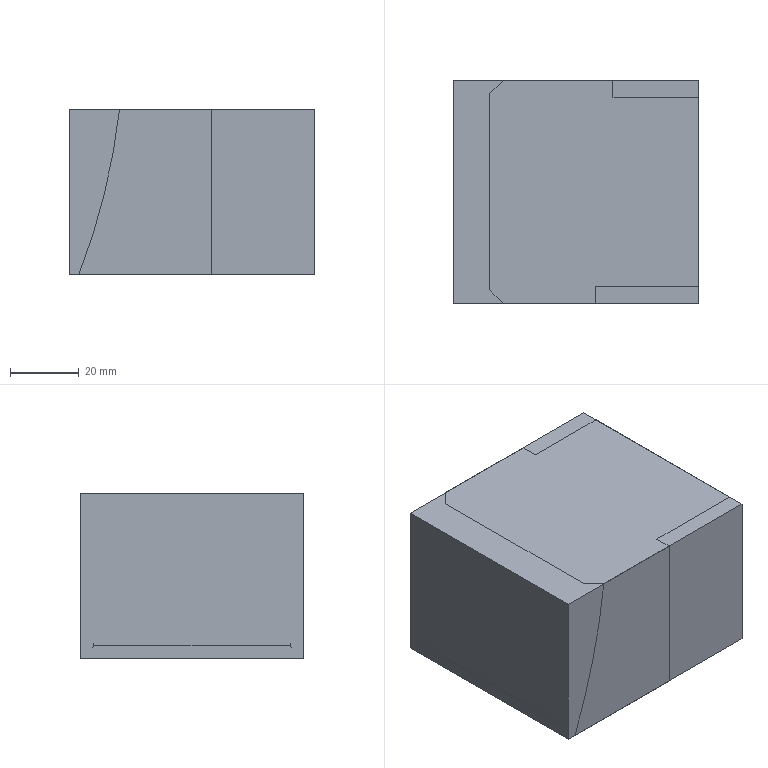NC program | NX | posted with a generic post | part box 71.51 x 65 x 48 mm
Lines 1 to 1113 of 48030:
N10 G17 G21 G94 G90
(FIXED_CONTOUR_COPY , TOOL : D6R0.5)
N12 T05 M6
N14 G54
N16 G17 G0 G90 X29.161 Y-29.75 B0. C0. S9500 M3
N18 G43 Z101.51 H5
N20 Z64.31
N22 G94 G1 Z60.474 F500.
N24 X29.148 Y-29.766
N26 X29.13 Y-29.777
N28 X29.109 Y-29.78
N30 X29.003 Z60.476 F3500.
N32 X28.925 Z60.478
N34 X28.771 Z60.481
N36 X28.616 Z60.482
N38 X28.46
N40 X27.842 Z60.481
N42 X-28.151
N44 X-28.306
N46 X-28.615 Z60.48
N48 X-28.77 Z60.479
N50 X-28.935 Z60.476
N52 X-28.999 Y-29.768
N54 X-29.072 Y-29.752
N56 X-29.124 Y-29.74
N58 X-29.079 Z60.477
N60 X-28.924 Z60.481
N62 X-28.77 Z60.483
N64 X-28.601 Z60.485
N66 X-28.306 Z60.486
N68 X-27.687
N70 X27.842
N72 X28.461 Z60.487
N74 X28.616
N76 X28.771 Z60.485
N78 X28.925 Z60.483
N80 X29.08 Z60.479
N82 X29.235 Z60.474
N84 X29.262 Z60.473
N86 X29.292 Y-29.731
N88 X29.388 Y-29.696
N90 X29.413 Y-29.687
N92 X29.389 Z60.475
N94 X29.235 Z60.481
N96 X29.08 Z60.485
N98 X28.925 Z60.489
N100 X28.771 Z60.491
N102 X28.616 Z60.493
N104 X28.461
N106 X27.842 Z60.492
N108 X-28.151
N110 X-28.306
N112 X-28.645 Z60.491
N114 X-28.77 Z60.489
N116 X-28.924 Z60.487
N118 X-29.079 Z60.483
N120 X-29.234 Z60.478
N122 X-29.306 Z60.476
N124 X-29.381 Y-29.661
N126 X-29.459 Y-29.631
N128 X-29.475 Y-29.624
N130 X-29.388 Z60.48
N132 X-29.234 Z60.486
N134 X-29.078 Z60.491
N136 X-28.924 Z60.494
N138 X-28.758 Z60.497
N140 X-28.652 Z60.498
N142 X-28.306 Z60.499
N144 X-25.977
N146 X27.842
N148 X28.461 Z60.5
N150 X28.616
N152 X28.771 Z60.499
N154 X28.931 Z60.496
N156 X29.086 Z60.493
N158 X29.234 Z60.488
N160 X29.389 Z60.482
N162 X29.544 Z60.474
N164 X29.569 Z60.473
N166 X29.691 Y-29.568
N168 X29.721 Y-29.552
N170 X29.699 Z60.474
N172 X29.544 Z60.483
N174 X29.389 Z60.49
N176 X29.235 Z60.496
N178 X29.08 Z60.501
N180 X28.925 Z60.505
N182 X28.771 Z60.507
N184 X28.616 Z60.509
N186 X28.461
N188 X27.842 Z60.508
N190 X-28.306
N192 X-28.619 Z60.507
N194 X-28.693 Z60.506
N196 X-28.77 Z60.505
N198 X-28.924 Z60.503
N200 X-29.079 Z60.499
N202 X-29.234 Z60.494
N204 X-29.388 Z60.488
N206 X-29.543 Z60.481
N208 X-29.635 Z60.476
N210 X-29.69 Y-29.524
N212 X-29.768 Y-29.482
N214 X-29.784 Y-29.472
N216 X-29.698 Z60.481
N218 X-29.542 Z60.49
N220 X-29.388 Z60.498
N222 X-29.234 Z60.504
N224 X-29.079 Z60.509
N226 X-28.924 Z60.512
N228 X-28.77 Z60.515
N230 X-28.657 Z60.516
N232 X-28.538
N234 X-28.46
N236 X-28.306 Z60.517
N238 X27.842
N240 X28.461 Z60.518
N242 X28.616
N244 X28.771 Z60.516
N246 X28.925 Z60.514
N248 X29.08 Z60.51
N250 X29.235 Z60.506
N252 X29.389 Z60.5
N254 X29.549 Z60.492
N256 X29.698 Z60.483
N258 X29.861 Z60.473
N260 X29.938 Y-29.422 Z60.472
N262 X29.988 Y-29.387 Z60.473
N264 X29.853 Z60.483
N266 X29.699 Z60.493
N268 X29.544 Z60.502
N270 X29.389 Z60.509
N272 X29.235 Z60.516
N274 X29.08 Z60.52
N276 X28.925 Z60.524
N278 X28.771 Z60.526
N280 X28.616 Z60.528
N282 X28.461
N284 X27.842 Z60.527
N286 X-28.306 Y-29.388
N288 X-28.46 Z60.526
N290 X-28.538
N292 X-28.655
N294 X-28.77 Z60.525
N296 X-28.924 Z60.522
N298 X-29.079 Z60.519
N300 X-29.234 Z60.514
N302 X-29.388 Z60.508
N304 X-29.543 Z60.5
N306 X-29.698 Z60.491
N308 X-29.852 Z60.481
N310 X-29.921 Z60.476
N312 X-29.935 Y-29.379
N314 X-30.002 Y-29.331
N316 X-30.046 Y-29.299
N318 X-30.007 Z60.479
N320 X-29.852 Z60.491
N322 X-29.698 Z60.502
N324 X-29.543 Z60.511
N326 X-29.388 Z60.518
N328 X-29.234 Z60.524
N330 X-29.079 Z60.529
N332 X-28.924 Z60.533
N334 X-28.77 Z60.535
N336 X-28.654 Z60.536
N338 X-28.541 Z60.537
N340 X-28.46
N342 X-28.311
N344 X27.838
N346 X28.461 Z60.538
N348 X28.616
N350 X28.771 Z60.537
N352 X28.925 Z60.534
N354 X29.08 Z60.531
N356 X29.235 Z60.526
N358 X29.389 Z60.52
N360 X29.544 Z60.513
N362 X29.699 Z60.504
N364 X29.853 Z60.493
N366 X30.008 Z60.481
N368 X30.114 Z60.472
N370 X30.157 Y-29.268 Z60.471
N372 X30.227 Y-29.206
N374 X30.163 Z60.478
N376 X30.008 Z60.492
N378 X29.853 Z60.504
N380 X29.699 Z60.514
N382 X29.544 Z60.523
N384 X29.389 Z60.531
N386 X29.235 Z60.537
N388 X29.08 Z60.541
N390 X28.925 Z60.545
N392 X28.771 Z60.548
N394 X28.616 Z60.549
N396 X28.461
N398 X27.842 Z60.548
N400 X-28.306 Y-29.207
N402 X-28.538
N404 X-28.657 Z60.547
N406 X-28.77 Z60.546
N408 X-28.924 Z60.544
N410 X-29.079 Z60.54
N412 X-29.234 Z60.535
N414 X-29.388 Z60.529
N416 X-29.543 Z60.522
N418 X-29.698 Z60.513
N420 X-29.852 Z60.502
N422 X-30.02 Z60.489
N424 X-30.163 Z60.476
N426 X-30.212 Y-29.164
N428 X-30.269 Y-29.112
N430 X-30.214 Z60.482
N432 X-30.162 Z60.487
N434 X-30.007 Z60.501
N436 X-29.852 Z60.513
N438 X-29.698 Z60.524
N440 X-29.543 Z60.533
N442 X-29.388 Z60.54
N444 X-29.234 Z60.546
N446 X-29.079 Z60.551
N448 X-28.924 Z60.555
N450 X-28.749 Z60.558
N452 X-28.62 Z60.559
N454 X-28.538
N456 X-28.151
N458 X27.842
N460 X28.152 Z60.56
N462 X28.461
N464 X28.616
N466 X28.771 Z60.559
N468 X28.925 Z60.556
N470 X29.08 Z60.552
N472 X29.235 Z60.548
N474 X29.389 Z60.542
N476 X29.544 Z60.534
N478 X29.699 Z60.525
N480 X29.853 Z60.515
N482 X30.008 Z60.503
N484 X30.163 Z60.489
N486 X30.298 Z60.475
N488 X30.333 Z60.47
N490 X30.4 Y-29.048
N492 X30.43 Y-29.016
N494 X30.314 Z60.484
N496 X30.163 Z60.5
N498 X30.008 Z60.514
N500 X29.853 Z60.526
N502 X29.699 Z60.537
N504 X29.544 Z60.545
N506 X29.389 Z60.553
N508 X29.235 Z60.559
N510 X29.08 Z60.564
N512 X28.925 Z60.567
N514 X28.771 Z60.57
N516 X28.616 Z60.571
N518 X28.461
N520 X27.997
N522 X27.201 Z60.57
N524 X-28.328
N526 X-28.538
N528 X-28.673
N530 X-28.77 Z60.569
N532 X-28.924 Z60.566
N534 X-29.079 Z60.562
N536 X-29.234 Z60.558
N538 X-29.388 Z60.552
N540 X-29.543 Z60.544
N542 X-29.698 Z60.535
N544 X-29.852 Z60.525
N546 X-30.007 Z60.513
N548 X-30.172 Z60.497
N550 X-30.316 Z60.482
N552 X-30.365 Z60.476
N554 X-30.408 Y-28.971
N556 X-30.42 Y-28.958
N558 X-30.454 Y-28.919
N560 X-30.355 Z60.488
N562 X-30.316 Z60.493
N564 X-30.162 Z60.51
N566 X-30.007 Z60.524
N568 X-29.852 Z60.536
N570 X-29.698 Z60.547
N572 X-29.543 Z60.556
N574 X-29.388 Z60.563
N576 X-29.234 Z60.569
N578 X-29.079 Z60.574
N580 X-28.924 Z60.578
N582 X-28.77 Z60.58
N584 X-28.62 Z60.581
N586 X-28.5 Z60.582
N588 X27.842
N590 X28.152
N592 X28.461 Z60.583
N594 X28.616 Z60.582
N596 X28.771 Z60.581
N598 X28.925 Z60.579
N600 X29.08 Z60.575
N602 X29.235 Z60.57
N604 X29.389 Z60.564
N606 X29.544 Z60.557
N608 X29.699 Z60.548
N610 X29.853 Z60.538
N612 X30.008 Z60.526
N614 X30.163 Z60.511
N616 X30.317 Z60.495
N618 X30.472 Z60.475
N620 X30.52 Z60.468
N622 X30.551 Y-28.883
N624 X30.586 Y-28.838
N626 X30.599 Y-28.821
N628 X30.582 Z60.471
N630 X30.472 Z60.487
N632 X30.317 Z60.506
N634 X30.163 Z60.523
N636 X30.008 Z60.537
N638 X29.853 Z60.549
N640 X29.699 Z60.559
N642 X29.544 Z60.568
N644 X29.389 Z60.576
N646 X29.235 Z60.582
N648 X29.08 Z60.586
N650 X28.925 Z60.59
N652 X28.771 Z60.592
N654 X28.616 Z60.594
N656 X28.461
N658 X27.997 Z60.593
N660 X27.087
N662 X-28.538
N664 X-28.659
N666 X-28.77 Z60.592
N668 X-28.924 Z60.589
N670 X-29.079 Z60.585
N672 X-29.234 Z60.581
N674 X-29.388 Z60.575
N676 X-29.543 Z60.567
N678 X-29.698 Z60.558
N680 X-29.852 Z60.548
N682 X-30.007 Z60.536
N684 X-30.162 Z60.521
N686 X-30.316 Z60.505
N688 X-30.471 Z60.485
N690 X-30.534 Z60.476
N692 X-30.55 Y-28.802
N694 X-30.609 Y-28.723
N696 X-30.572 Z60.482
N698 X-30.471 Z60.497
N700 X-30.316 Z60.516
N702 X-30.162 Z60.533
N704 X-30.007 Z60.547
N706 X-29.852 Z60.559
N708 X-29.698 Z60.57
N710 X-29.543 Z60.579
N712 X-29.388 Z60.586
N714 X-29.234 Z60.592
N716 X-29.079 Z60.597
N718 X-28.924 Z60.601
N720 X-28.77 Z60.603
N722 X-28.657 Z60.604
N724 X-28.538 Z60.605
N726 X-27.687
N728 X27.842
N730 X28.461 Z60.606
N732 X28.616 Z60.605
N734 X28.771 Z60.604
N736 X28.925 Z60.601
N738 X29.08 Z60.598
N740 X29.235 Z60.593
N742 X29.389 Z60.587
N744 X29.544 Z60.58
N746 X29.699 Z60.571
N748 X29.853 Z60.561
N750 X30.008 Z60.548
N752 X30.163 Z60.534
N754 X30.317 Z60.518
N756 X30.472 Z60.498
N758 X30.558 Z60.486
N760 X30.627 Z60.475
N762 X30.674 Z60.467
N764 X30.707 Y-28.68 Z60.466
N766 X30.73 Y-28.649 Z60.465
N768 X30.748 Y-28.624 Z60.464
N770 X30.704 Z60.473
N772 X30.627 Z60.487
N774 X30.549 Z60.499
N776 X30.472 Z60.51
N778 X30.317 Z60.529
N780 X30.163 Z60.546
N782 X30.008 Z60.56
N784 X29.853 Z60.572
N786 X29.699 Z60.582
N788 X29.544 Z60.591
N790 X29.389 Z60.599
N792 X29.235 Z60.605
N794 X29.08 Z60.609
N796 X28.925 Z60.613
N798 X28.771 Z60.615
N800 X28.616 Z60.617
N802 X28.461
N804 X27.842 Z60.616
N806 X-28.151 Y-28.625
N808 X-28.538 Z60.617
N810 X-28.66 Z60.616
N812 X-28.77 Z60.615
N814 X-28.924 Z60.612
N816 X-29.079 Z60.609
N818 X-29.234 Z60.604
N820 X-29.388 Z60.598
N822 X-29.543 Z60.59
N824 X-29.698 Z60.581
N826 X-29.852 Z60.571
N828 X-30.007 Z60.559
N830 X-30.162 Z60.545
N832 X-30.316 Z60.528
N834 X-30.471 Z60.508
N836 X-30.549 Z60.497
N838 X-30.626 Z60.485
N840 X-30.677 Z60.476
N842 X-30.71 Y-28.572
N844 X-30.739 Y-28.526
N846 X-30.668 Z60.489
N848 X-30.626 Z60.496
N850 X-30.549 Z60.509
N852 X-30.471 Z60.52
N854 X-30.316 Z60.54
N856 X-30.162 Z60.556
N858 X-30.007 Z60.57
N860 X-29.852 Z60.583
N862 X-29.698 Z60.593
N864 X-29.543 Z60.602
N866 X-29.388 Z60.609
N868 X-29.234 Z60.616
N870 X-29.079 Z60.62
N872 X-28.924 Z60.624
N874 X-28.77 Z60.627
N876 X-28.658 Z60.628
N878 X-28.54
N880 X-27.687
N882 X27.842
N884 X28.461 Z60.629
N886 X28.616 Z60.628
N888 X28.771 Z60.627
N890 X28.925 Z60.625
N892 X29.08 Z60.621
N894 X29.235 Z60.616
N896 X29.389 Z60.61
N898 X29.544 Z60.603
N900 X29.699 Z60.594
N902 X29.853 Z60.584
N904 X30.008 Z60.571
N906 X30.163 Z60.557
N908 X30.317 Z60.541
N910 X30.472 Z60.521
N912 X30.549 Z60.51
N914 X30.627 Z60.498
N916 X30.704 Z60.485
N918 X30.781 Z60.469
N920 X30.813 Z60.463
N922 X30.833 Y-28.494 Z60.461
N924 X30.875 Y-28.427 Z60.459
N926 X30.833 Z60.47
N928 X30.781 Z60.481
N930 X30.704 Z60.496
N932 X30.627 Z60.51
N934 X30.549 Z60.522
N936 X30.472 Z60.533
N938 X30.317 Z60.552
N940 X30.163 Z60.569
N942 X30.008 Z60.583
N944 X29.853 Z60.595
N946 X29.699 Z60.605
N948 X29.544 Z60.614
N950 X29.389 Z60.622
N952 X29.235 Z60.628
N954 X29.08 Z60.632
N956 X28.925 Z60.636
N958 X28.771 Z60.639
N960 X28.616 Z60.64
N962 X28.461
N964 X27.842 Z60.639
N966 X-27.944
N968 X-28.46 Z60.64
N970 X-28.619
N972 X-28.77 Z60.638
N974 X-28.924 Z60.636
N976 X-29.079 Z60.632
N978 X-29.234 Z60.627
N980 X-29.388 Z60.621
N982 X-29.543 Z60.614
N984 X-29.698 Z60.605
N986 X-29.852 Z60.594
N988 X-30.007 Z60.582
N990 X-30.162 Z60.568
N992 X-30.316 Z60.551
N994 X-30.471 Z60.532
N996 X-30.549 Z60.52
N998 X-30.626 Z60.508
N1000 X-30.7 Z60.495
N1002 X-30.778 Z60.48
N1004 X-30.795 Z60.476
N1006 X-30.842 Y-28.339
N1008 X-30.848 Y-28.328
N1010 X-30.781 Z60.491
N1012 X-30.703 Z60.506
N1014 X-30.626 Z60.52
N1016 X-30.549 Z60.532
N1018 X-30.471 Z60.543
N1020 X-30.316 Z60.563
N1022 X-30.162 Z60.58
N1024 X-30.007 Z60.594
N1026 X-29.852 Z60.606
N1028 X-29.698 Z60.617
N1030 X-29.543 Z60.625
N1032 X-29.388 Z60.633
N1034 X-29.234 Z60.639
N1036 X-29.079 Z60.644
N1038 X-28.924 Z60.647
N1040 X-28.77 Z60.65
N1042 X-28.615 Z60.651
N1044 X-28.413
N1046 X-27.949
N1048 X27.842
N1050 X28.461 Z60.652
N1052 X28.616 Z60.651
N1054 X28.771 Z60.65
N1056 X28.925 Z60.648
N1058 X29.08 Z60.644
N1060 X29.235 Z60.639
N1062 X29.389 Z60.633
N1064 X29.544 Z60.626
N1066 X29.699 Z60.617
N1068 X29.853 Z60.607
N1070 X30.008 Z60.595
N1072 X30.163 Z60.58
N1074 X30.317 Z60.564
N1076 X30.472 Z60.544
N1078 X30.549 Z60.533
N1080 X30.627 Z60.521
N1082 X30.704 Z60.508
N1084 X30.781 Z60.492
N1086 X30.849 Z60.478
N1088 X30.892 Z60.467
N1090 X30.934 Z60.456
N1092 X30.989 Y-28.228 Z60.451
N1094 X30.934 Z60.468
N1096 X30.858 Z60.487
N1098 X30.781 Z60.504
N1100 X30.704 Z60.519
N1102 X30.627 Z60.533
N1104 X30.549 Z60.545
N1106 X30.472 Z60.556
N1108 X30.317 Z60.576
N1110 X30.163 Z60.592
N1112 X30.008 Z60.606
N1114 X29.853 Z60.618
N1116 X29.699 Z60.629
N1118 X29.544 Z60.637
N1120 X29.389 Z60.645
N1122 X29.235 Z60.651
N1124 X29.08 Z60.656
N1126 X28.925 Z60.659
N1128 X28.771 Z60.662
N1130 X28.616 Z60.663
N1132 X28.461
N1134 X27.997
N1136 X-28.005
N1138 X-28.46
N1140 X-28.615
N1142 X-28.77 Z60.661
N1144 X-28.924 Z60.659
N1146 X-29.079 Z60.655
N1148 X-29.234 Z60.651
N1150 X-29.388 Z60.644
N1152 X-29.543 Z60.637
N1154 X-29.698 Z60.628
N1156 X-29.852 Z60.618
N1158 X-29.955 Z60.61
N1160 X-30.007 Z60.606
N1162 X-30.162 Z60.591
N1164 X-30.316 Z60.575
N1166 X-30.471 Z60.555
N1168 X-30.549 Z60.544
N1170 X-30.626 Z60.531
N1172 X-30.703 Z60.518
N1174 X-30.781 Z60.502
N1176 X-30.81 Z60.496
N1178 X-30.816 Z60.495
N1180 X-30.856 Z60.485
N1182 X-30.896 Z60.476
N1184 X-30.916 Y-28.185
N1186 X-30.929 Y-28.154
N1188 X-30.939 Y-28.129
N1190 X-30.863 Z60.496
N1192 X-30.851 Z60.499
N1194 X-30.781 Z60.514
N1196 X-30.703 Z60.529
N1198 X-30.626 Z60.543
N1200 X-30.549 Z60.555
N1202 X-30.471 Z60.567
N1204 X-30.316 Z60.586
N1206 X-30.162 Z60.603
N1208 X-30.007 Z60.617
N1210 X-29.9 Z60.626
N1212 X-29.796 Z60.633
N1214 X-29.698 Z60.64
N1216 X-29.543 Z60.649
N1218 X-29.388 Z60.656
N1220 X-29.234 Z60.662
N1222 X-29.079 Z60.667
N1224 X-28.924 Z60.671
N1226 X-28.77 Z60.673
N1228 X-28.615 Z60.674
N1230 X-28.46 Z60.675
N1232 X-27.906 Z60.674
N1234 X27.997
N1236 X28.461 Z60.675
N1238 X28.616
N1240 X28.771 Z60.673
N1242 X28.925 Z60.671
N1244 X29.08 Z60.667
N1246 X29.235 Z60.662
N1248 X29.389 Z60.656
N1250 X29.544 Z60.649
N1252 X29.699 Z60.64
N1254 X29.853 Z60.63
N1256 X30.008 Z60.618
N1258 X30.163 Z60.604
N1260 X30.317 Z60.587
N1262 X30.472 Z60.568
N1264 X30.549 Z60.557
N1266 X30.627 Z60.544
N1268 X30.704 Z60.531
N1270 X30.781 Z60.516
N1272 X30.859 Z60.498
N1274 X30.936 Z60.479
N1276 X31.002 Z60.459
N1278 X31.033 Z60.449
N1280 X31.043 Z60.445
N1282 X31.078 Y-28.065 Z60.44
N1284 X31.091 Y-28.041 Z60.437
N1286 X31.097 Y-28.03 Z60.436
N1288 X31.091 Z60.439
N1290 X31.081 Z60.443
N1292 X31.045 Z60.456
N1294 X31.008 Z60.469
N1296 X30.936 Z60.49
N1298 X30.859 Z60.51
N1300 X30.781 Z60.527
N1302 X30.704 Z60.542
N1304 X30.627 Z60.556
N1306 X30.549 Z60.568
N1308 X30.472 Z60.579
N1310 X30.317 Z60.599
N1312 X30.163 Z60.615
N1314 X30.008 Z60.629
N1316 X29.853 Z60.641
N1318 X29.699 Z60.652
N1320 X29.544 Z60.661
N1322 X29.389 Z60.668
N1324 X29.235 Z60.674
N1326 X29.08 Z60.679
N1328 X28.925 Z60.682
N1330 X28.771 Z60.685
N1332 X28.616 Z60.686
N1334 X28.461
N1336 X27.842
N1338 X-27.996
N1340 X-28.46
N1342 X-28.615
N1344 X-28.77 Z60.685
N1346 X-28.924 Z60.682
N1348 X-29.079 Z60.679
N1350 X-29.234 Z60.674
N1352 X-29.388 Z60.668
N1354 X-29.543 Z60.66
N1356 X-29.698 Z60.652
N1358 X-29.796 Z60.645
N1360 X-29.877 Z60.639
N1362 X-29.97 Z60.632
N1364 X-30.007 Z60.629
N1366 X-30.162 Z60.615
N1368 X-30.316 Z60.598
N1370 X-30.471 Z60.578
N1372 X-30.549 Z60.567
N1374 X-30.626 Z60.555
N1376 X-30.703 Z60.541
N1378 X-30.781 Z60.526
N1380 X-30.858 Z60.509
N1382 X-30.935 Z60.489
N1384 X-30.979 Z60.476
N1386 X-31.015 Y-27.931
N1388 X-30.973 Z60.489
N1390 X-30.946 Z60.497
N1392 X-30.935 Z60.5
N1394 X-30.858 Z60.52
N1396 X-30.781 Z60.538
N1398 X-30.703 Z60.553
N1400 X-30.626 Z60.567
N1402 X-30.549 Z60.579
N1404 X-30.471 Z60.59
N1406 X-30.316 Z60.61
N1408 X-30.162 Z60.626
N1410 X-30.001 Z60.641
N1412 X-29.852 Z60.653
N1414 X-29.723 Z60.662
N1416 X-29.698 Z60.663
N1418 X-29.543 Z60.672
N1420 X-29.388 Z60.679
N1422 X-29.234 Z60.685
N1424 X-29.079 Z60.69
N1426 X-28.924 Z60.694
N1428 X-28.77 Z60.696
N1430 X-28.615 Z60.698
N1432 X-28.46
N1434 X-27.862 Z60.697
N1436 X27.977 Z60.698
N1438 X28.461
N1440 X28.616
N1442 X28.771 Z60.696
N1444 X28.925 Z60.694
N1446 X29.08 Z60.69
N1448 X29.235 Z60.685
N1450 X29.389 Z60.679
N1452 X29.544 Z60.672
N1454 X29.699 Z60.663
N1456 X29.853 Z60.653
N1458 X30.008 Z60.641
N1460 X30.163 Z60.627
N1462 X30.317 Z60.61
N1464 X30.472 Z60.591
N1466 X30.549 Z60.58
N1468 X30.627 Z60.567
N1470 X30.704 Z60.554
N1472 X30.781 Z60.539
N1474 X30.859 Z60.522
N1476 X30.936 Z60.502
N1478 X31.013 Z60.479
N1480 X31.051 Z60.466
N1482 X31.091 Z60.45
N1484 X31.121 Z60.437
N1486 X31.151 Z60.423
N1488 X31.162 Y-27.91 Z60.42
N1490 X31.173 Y-27.891 Z60.417
N1492 X31.181 Y-27.876 Z60.414
N1494 X31.207 Y-27.831 Z60.404
N1496 X31.188 Z60.415
N1498 X31.165 Z60.428
N1500 X31.128 Z60.446
N1502 X31.091 Z60.462
N1504 X31.052 Z60.477
N1506 X31.013 Z60.49
N1508 X30.936 Z60.513
N1510 X30.859 Z60.533
N1512 X30.781 Z60.55
N1514 X30.704 Z60.566
N1516 X30.627 Z60.579
N1518 X30.549 Z60.591
N1520 X30.472 Z60.602
N1522 X30.317 Z60.622
N1524 X30.163 Z60.638
N1526 X30.008 Z60.652
N1528 X29.853 Z60.665
N1530 X29.699 Z60.675
N1532 X29.544 Z60.684
N1534 X29.389 Z60.691
N1536 X29.235 Z60.697
N1538 X29.08 Z60.702
N1540 X28.925 Z60.705
N1542 X28.771 Z60.708
N1544 X28.616 Z60.709
N1546 X28.461 Z60.71
N1548 X27.767 Z60.709
N1550 X-27.996
N1552 X-28.46
N1554 X-28.615
N1556 X-28.77 Z60.708
N1558 X-28.924 Z60.705
N1560 X-29.079 Z60.702
N1562 X-29.234 Z60.697
N1564 X-29.388 Z60.691
N1566 X-29.543 Z60.684
N1568 X-29.698 Z60.675
N1570 X-29.852 Z60.664
N1572 X-30.007 Z60.652
N1574 X-30.162 Z60.638
N1576 X-30.316 Z60.621
N1578 X-30.471 Z60.602
N1580 X-30.549 Z60.591
N1582 X-30.626 Z60.578
N1584 X-30.703 Z60.565
N1586 X-30.781 Z60.549
N1588 X-30.858 Z60.532
N1590 X-30.935 Z60.512
N1592 X-31.013 Z60.489
N1594 X-31.049 Z60.476
N1596 X-31.073 Y-27.754
N1598 X-31.08 Y-27.732
N1600 X-31.056 Z60.485
N1602 X-31.027 Z60.496
N1604 X-31.013 Z60.5
N1606 X-30.935 Z60.524
N1608 X-30.858 Z60.544
N1610 X-30.781 Z60.561
N1612 X-30.703 Z60.576
N1614 X-30.626 Z60.59
N1616 X-30.549 Z60.602
N1618 X-30.471 Z60.613
N1620 X-30.316 Z60.633
N1622 X-30.162 Z60.65
N1624 X-30.007 Z60.664
N1626 X-29.852 Z60.676
N1628 X-29.698 Z60.686
N1630 X-29.543 Z60.695
N1632 X-29.388 Z60.702
N1634 X-29.234 Z60.709
N1636 X-29.079 Z60.713
N1638 X-28.924 Z60.717
N1640 X-28.77 Z60.719
N1642 X-28.615 Z60.721
N1644 X-28.46
N1646 X-27.664
N1648 X27.974
N1650 X28.461
N1652 X28.616
N1654 X28.771 Z60.719
N1656 X28.925 Z60.717
N1658 X29.08 Z60.713
N1660 X29.235 Z60.709
N1662 X29.389 Z60.703
N1664 X29.544 Z60.695
N1666 X29.699 Z60.686
N1668 X29.853 Z60.676
N1670 X30.008 Z60.664
N1672 X30.163 Z60.65
N1674 X30.317 Z60.633
N1676 X30.472 Z60.614
N1678 X30.549 Z60.603
N1680 X30.627 Z60.591
N1682 X30.704 Z60.577
N1684 X30.781 Z60.562
N1686 X30.859 Z60.545
N1688 X30.936 Z60.525
N1690 X31.013 Z60.502
N1692 X31.052 Z60.488
N1694 X31.091 Z60.473
N1696 X31.129 Z60.457
N1698 X31.168 Z60.438
N1700 X31.207 Z60.417
N1702 X31.245 Z60.392
N1704 X31.251 Z60.388
N1706 X31.268 Z60.376
N1708 X31.275 Y-27.721 Z60.372
N1710 X31.295 Y-27.69 Z60.359
N1712 X31.318 Y-27.655 Z60.343
N1714 X31.332 Y-27.633 Z60.332
N1716 X31.32 Z60.344
N1718 X31.3 Z60.361
N1720 X31.281 Z60.377
N1722 X31.245 Z60.403
N1724 X31.207 Z60.428
N1726 X31.168 Z60.449
N1728 X31.129 Z60.468
N1730 X31.091 Z60.485
N1732 X31.052 Z60.5
N1734 X31.013 Z60.513
N1736 X30.936 Z60.537
N1738 X30.859 Z60.556
N1740 X30.781 Z60.573
N1742 X30.704 Z60.589
N1744 X30.627 Z60.602
N1746 X30.549 Z60.614
N1748 X30.472 Z60.625
N1750 X30.317 Z60.645
N1752 X30.163 Z60.661
N1754 X30.008 Z60.676
N1756 X29.853 Z60.688
N1758 X29.699 Z60.698
N1760 X29.544 Z60.707
N1762 X29.389 Z60.714
N1764 X29.235 Z60.72
N1766 X29.08 Z60.725
N1768 X28.925 Z60.729
N1770 X28.771 Z60.731
N1772 X28.616 Z60.732
N1774 X28.461 Z60.733
N1776 X27.81 Z60.732
N1778 X-28.029
N1780 X-28.46 Z60.733
N1782 X-28.615 Z60.732
N1784 X-28.77 Z60.731
N1786 X-28.924 Z60.728
N1788 X-29.079 Z60.725
N1790 X-29.234 Z60.72
N1792 X-29.388 Z60.714
N1794 X-29.543 Z60.707
N1796 X-29.698 Z60.698
N1798 X-29.852 Z60.688
N1800 X-30.007 Z60.675
N1802 X-30.162 Z60.661
N1804 X-30.316 Z60.645
N1806 X-30.471 Z60.625
N1808 X-30.549 Z60.614
N1810 X-30.626 Z60.602
N1812 X-30.703 Z60.588
N1814 X-30.781 Z60.573
N1816 X-30.858 Z60.555
N1818 X-30.935 Z60.535
N1820 X-31.013 Z60.512
N1822 X-31.052 Z60.498
N1824 X-31.09 Z60.484
N1826 X-31.109 Z60.476
N1828 X-31.112 Y-27.622 Z60.475
N1830 X-31.114
N1832 X-31.14 Z60.463
N1834 X-31.171 Z60.448
N1836 X-31.192 Z60.436
N1838 X-31.21 Y-27.621 Z60.426
N1840 X-31.225 Z60.416
N1842 X-31.245 Z60.403
N1844 X-31.277 Y-27.62 Z60.38
N1846 X-31.283 Z60.375
N1848 X-31.303 Z60.359
N1850 X-31.314 Y-27.619 Z60.349
N1852 X-31.322 Y-27.62 Z60.342
N1854 X-31.333 Z60.331
N1856 X-31.352 Y-27.624 Z60.311
N1858 X-31.399 Y-27.623 Z60.265
N1860 X-31.554 Y-27.62 Z60.11
N1862 X-31.709 Y-27.618 Z59.955
N1864 X-31.863 Y-27.617 Z59.8
N1866 X-32.018 Y-27.616 Z59.644
N1868 X-32.656 Z59.002
N1870 X-32.938 Z58.719
N1872 X-33.151 Y-27.614 Z58.505
N1874 X-33.255 Z58.402
N1876 X-33.41 Y-27.613 Z58.247
N1878 X-33.719 Z57.936
N1880 X-34.493 Z57.157
N1882 X-34.803 Y-27.612 Z56.845
N1884 X-34.957 Y-27.611 Z56.691
N1886 X-37.661 Y-27.592 Z53.973
N1888 Y-27.534 Z53.98
N1890 X-34.714 Z56.944
N1892 X-33.565 Z58.101
N1894 X-33.41 Z58.256
N1896 X-33.255 Z58.411
N1898 X-32.946 Z58.72
N1900 X-32.637 Z59.031
N1902 X-31.554 Z60.12
N1904 X-31.399 Z60.275
N1906 X-31.322 Z60.352
N1908 X-31.303 Z60.369
N1910 X-31.283 Z60.385
N1912 X-31.245 Z60.414
N1914 X-31.206 Z60.438
N1916 X-31.167 Z60.46
N1918 X-31.154 Z60.466
N1920 X-31.129 Z60.479
N1922 X-31.09 Z60.495
N1924 X-31.051 Z60.51
N1926 X-31.013 Z60.524
N1928 X-30.935 Z60.547
N1930 X-30.858 Z60.567
N1932 X-30.781 Z60.584
N1934 X-30.703 Z60.6
N1936 X-30.626 Z60.613
N1938 X-30.549 Z60.626
N1940 X-30.471 Z60.637
N1942 X-30.316 Z60.656
N1944 X-30.162 Z60.673
N1946 X-30.007 Z60.687
N1948 X-29.852 Z60.699
N1950 X-29.698 Z60.709
N1952 X-29.543 Z60.718
N1954 X-29.388 Z60.726
N1956 X-29.234 Z60.732
N1958 X-29.079 Z60.736
N1960 X-28.924 Z60.74
N1962 X-28.77 Z60.743
N1964 X-28.615 Z60.744
N1966 X-28.46
N1968 X-27.687
N1970 X28.152
N1972 X28.461
N1974 X28.616
N1976 X28.771 Z60.743
N1978 X28.925 Z60.74
N1980 X29.08 Z60.736
N1982 X29.235 Z60.732
N1984 X29.389 Z60.726
N1986 X29.544 Z60.718
N1988 X29.699 Z60.71
N1990 X29.853 Z60.699
N1992 X30.008 Z60.687
N1994 X30.163 Z60.673
N1996 X30.317 Z60.657
N1998 X30.472 Z60.637
N2000 X30.549 Z60.626
N2002 X30.627 Z60.614
N2004 X30.704 Z60.6
N2006 X30.781 Z60.585
N2008 X30.859 Z60.568
N2010 X30.936 Z60.548
N2012 X31.013 Z60.525
N2014 X31.052 Z60.511
N2016 X31.091 Z60.496
N2018 X31.129 Z60.48
N2020 X31.168 Z60.461
N2022 X31.207 Z60.44
N2024 X31.245 Z60.415
N2026 X31.284 Z60.387
N2028 X31.303 Z60.371
N2030 X31.323 Z60.353
N2032 X31.4 Z60.276
N2034 X31.709 Z59.965
N2036 X32.792 Z58.876
N2038 X33.013 Z58.654
N2040 X33.256 Z58.411
N2042 X33.411 Z58.256
N2044 X33.72 Z57.945
N2046 X34.803 Z56.855
N2048 X37.662 Z53.98
N2050 Y-27.435 Z53.992
N2052 X34.648 Z57.022
N2054 X33.566 Z58.112
N2056 X33.411 Z58.267
N2058 X33.256 Z58.422
N2060 X32.947 Z58.732
N2062 X32.638 Z59.043
N2064 X31.555 Z60.132
N2066 X31.4 Z60.288
N2068 X31.323 Z60.365
N2070 X31.303 Z60.382
N2072 X31.284 Z60.398
N2074 X31.245 Z60.427
N2076 X31.207 Z60.451
N2078 X31.168 Z60.473
N2080 X31.129 Z60.491
N2082 X31.091 Z60.508
N2084 X31.052 Z60.523
N2086 X31.013 Z60.536
N2088 X30.936 Z60.56
N2090 X30.859 Z60.579
N2092 X30.781 Z60.597
N2094 X30.704 Z60.612
N2096 X30.627 Z60.625
N2098 X30.549 Z60.638
N2100 X30.472 Z60.649
N2102 X30.317 Z60.668
N2104 X30.163 Z60.685
N2106 X30.008 Z60.699
N2108 X29.853 Z60.711
N2110 X29.699 Z60.721
N2112 X29.544 Z60.73
N2114 X29.389 Z60.737
N2116 X29.235 Z60.743
N2118 X29.08 Z60.748
N2120 X28.925 Z60.752
N2122 X28.771 Z60.754
N2124 X28.616 Z60.756
N2126 X28.461
N2128 X27.688
N2130 X-28.151
N2132 X-28.46
N2134 X-28.615
N2136 X-28.77 Z60.754
N2138 X-28.924 Z60.752
N2140 X-29.079 Z60.748
N2142 X-29.234 Z60.743
N2144 X-29.388 Z60.737
N2146 X-29.543 Z60.73
N2148 X-29.698 Z60.721
N2150 X-29.852 Z60.711
N2152 X-30.007 Z60.699
N2154 X-30.162 Z60.684
N2156 X-30.316 Z60.668
N2158 X-30.471 Z60.648
N2160 X-30.549 Z60.637
N2162 X-30.626 Z60.625
N2164 X-30.703 Z60.611
N2166 X-30.781 Z60.596
N2168 X-30.858 Z60.579
N2170 X-30.935 Z60.559
N2172 X-31.013 Z60.535
N2174 X-31.051 Z60.522
N2176 X-31.09 Z60.507
N2178 X-31.129 Z60.49
N2180 X-31.167 Z60.471
N2182 X-31.206 Z60.45
N2184 X-31.245 Z60.425
N2186 X-31.283 Z60.397
N2188 X-31.303 Z60.381
N2190 X-31.322 Z60.364
N2192 X-31.399 Z60.287
N2194 X-31.554 Z60.132
N2196 X-32.791 Z58.887
N2198 X-32.946 Z58.731
N2200 X-33.41 Z58.267
N2202 X-33.73 Z57.945
N2204 X-34.968 Z56.7
N2206 X-37.661 Z53.991
N2208 X-37.662 Y-27.335 Z54.002
N2210 X-34.758 Z56.923
N2212 X-33.565 Z58.124
N2214 X-33.41 Z58.279
N2216 X-32.946 Z58.743
N2218 X-32.637 Z59.054
N2220 X-31.554 Z60.143
N2222 X-31.399 Z60.299
N2224 X-31.322 Z60.375